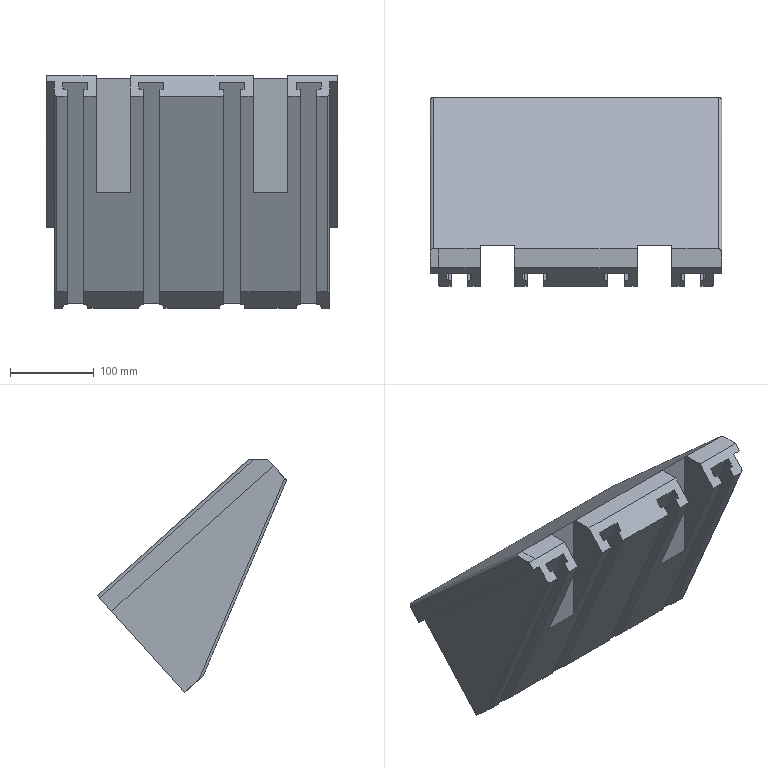Part | Creo | 1 solid | 71 faces | box 348.804 x 225.783 x 278.414 mm | volume 8478569 mm3 | plane 59 | cylinder 12 | commonest cylinder face diameters 4 x6 2 x2 6 x2 8 x2